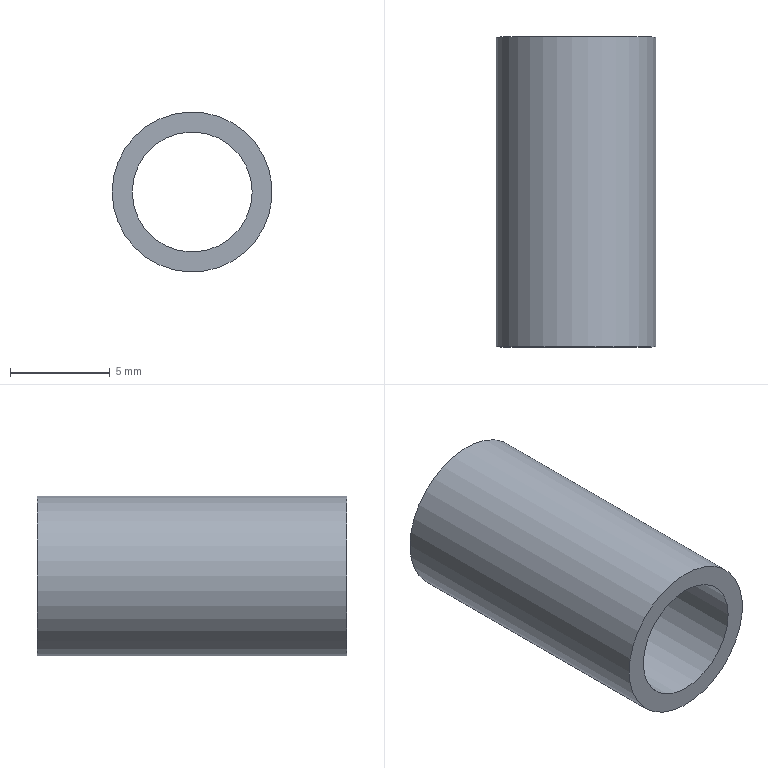Part | STEP file | 1-41.4 | 1 solid | 4 faces | box 8 x 15.5 x 8 mm | volume 340.863 mm3 | plane 2 | cylinder 2 | commonest cylinder face diameters 6 x1 8 x1
STEP:
#1=CARTESIAN_POINT('',(0.,0.,0.));
#2=DIRECTION('',(0.,0.,1.));
#3=DIRECTION('',(1.,0.,0.));
#4=AXIS2_PLACEMENT_3D('',#1,#2,#3);
#5=CARTESIAN_POINT('',(-4.,0.,0.));
#6=VERTEX_POINT('',#5);
#7=CARTESIAN_POINT('',(0.,0.,0.));
#8=DIRECTION('',(0.,1.,0.));
#9=DIRECTION('',(-1.,0.,0.));
#10=AXIS2_PLACEMENT_3D('',#7,#8,#9);
#11=CIRCLE('',#10,4.);
#12=CARTESIAN_POINT('',(1.072,0.,0.));
#13=DIRECTION('',(0.,1.,0.));
#14=DIRECTION('',(-1.,0.,0.));
#15=AXIS2_PLACEMENT_3D('',#12,#13,#14);
#16=PLANE('',#15);
#17=CARTESIAN_POINT('',(1.072,0.));
#18=DIRECTION('',(1.,0.));
#19=AXIS2_PLACEMENT_2D('',#17,#18);
#20=CIRCLE('',#19,4.);
#21=(GEOMETRIC_REPRESENTATION_CONTEXT(2)PARAMETRIC_REPRESENTATION_CONTEXT()REPRESENTATION_CONTEXT('',''));
#22=DEFINITIONAL_REPRESENTATION('',(#20),#21);
#23=PCURVE('',#16,#22);
#24=CARTESIAN_POINT('',(0.,0.,0.));
#25=DIRECTION('',(0.,-1.,0.));
#26=DIRECTION('',(-1.,0.,0.));
#27=AXIS2_PLACEMENT_3D('',#24,#25,#26);
#28=CYLINDRICAL_SURFACE('',#27,4.);
#29=CARTESIAN_POINT('',(6.283,0.));
#30=DIRECTION('',(-1.,0.));
#31=VECTOR('',#30,1.);
#32=LINE('',#29,#31);
#33=(GEOMETRIC_REPRESENTATION_CONTEXT(2)PARAMETRIC_REPRESENTATION_CONTEXT()REPRESENTATION_CONTEXT('',''));
#34=DEFINITIONAL_REPRESENTATION('',(#32),#33);
#35=PCURVE('',#28,#34);
#36=SURFACE_CURVE('',#11,(#23,#35),.PCURVE_S1.);
#37=EDGE_CURVE('',#6,#6,#36,.T.);
#38=ORIENTED_EDGE('',*,*,#37,.T.);
#39=EDGE_LOOP('',(#38));
#40=FACE_BOUND('',#39,.T.);
#41=CARTESIAN_POINT('',(-3.,0.,0.));
#42=VERTEX_POINT('',#41);
#43=CARTESIAN_POINT('',(0.,0.,0.));
#44=DIRECTION('',(0.,-1.,0.));
#45=DIRECTION('',(-1.,0.,0.));
#46=AXIS2_PLACEMENT_3D('',#43,#44,#45);
#47=CIRCLE('',#46,3.);
#48=CARTESIAN_POINT('',(4.072,0.));
#49=CARTESIAN_POINT('',(4.072,-5.196));
#50=CARTESIAN_POINT('',(-0.4282,-2.598));
#51=CARTESIAN_POINT('',(-4.928,0.));
#52=CARTESIAN_POINT('',(-0.4282,2.598));
#53=CARTESIAN_POINT('',(4.072,5.196));
#54=CARTESIAN_POINT('',(4.072,0.));
#55=(BOUNDED_CURVE()B_SPLINE_CURVE(2,(#48,#49,#50,#51,#52,#53,#54),.UNSPECIFIED.,.T.,.F.)B_SPLINE_CURVE_WITH_KNOTS((1,2,2,2,2,1),(-2.094,0.,2.094,4.189,6.283,8.378),.UNSPECIFIED.)CURVE()GEOMETRIC_REPRESENTATION_ITEM()RATIONAL_B_SPLINE_CURVE((1.,0.5,1.,0.5,1.,0.5,1.))REPRESENTATION_ITEM(''));
#56=(GEOMETRIC_REPRESENTATION_CONTEXT(2)PARAMETRIC_REPRESENTATION_CONTEXT()REPRESENTATION_CONTEXT('',''));
#57=DEFINITIONAL_REPRESENTATION('',(#55),#56);
#58=PCURVE('',#16,#57);
#59=CARTESIAN_POINT('',(0.,0.,0.));
#60=DIRECTION('',(0.,-1.,0.));
#61=DIRECTION('',(-1.,0.,0.));
#62=AXIS2_PLACEMENT_3D('',#59,#60,#61);
#63=CYLINDRICAL_SURFACE('',#62,3.);
#64=CARTESIAN_POINT('',(0.,0.));
#65=DIRECTION('',(1.,0.));
#66=VECTOR('',#65,1.);
#67=LINE('',#64,#66);
#68=(GEOMETRIC_REPRESENTATION_CONTEXT(2)PARAMETRIC_REPRESENTATION_CONTEXT()REPRESENTATION_CONTEXT('',''));
#69=DEFINITIONAL_REPRESENTATION('',(#67),#68);
#70=PCURVE('',#63,#69);
#71=SURFACE_CURVE('',#47,(#58,#70),.PCURVE_S1.);
#72=EDGE_CURVE('',#42,#42,#71,.T.);
#73=ORIENTED_EDGE('',*,*,#72,.T.);
#74=EDGE_LOOP('',(#73));
#75=FACE_BOUND('',#74,.T.);
#76=ADVANCED_FACE('',(#40,#75),#16,.T.);
#77=CARTESIAN_POINT('',(-4.,-15.5,0.));
#78=VERTEX_POINT('',#77);
#79=CARTESIAN_POINT('',(0.,-15.5,0.));
#80=DIRECTION('',(0.,1.,0.));
#81=DIRECTION('',(-1.,0.,0.));
#82=AXIS2_PLACEMENT_3D('',#79,#80,#81);
#83=CIRCLE('',#82,4.);
#84=CARTESIAN_POINT('',(1.072,-15.5,0.));
#85=DIRECTION('',(0.,1.,0.));
#86=DIRECTION('',(-1.,0.,0.));
#87=AXIS2_PLACEMENT_3D('',#84,#85,#86);
#88=PLANE('',#87);
#89=CARTESIAN_POINT('',(1.072,0.));
#90=DIRECTION('',(1.,0.));
#91=AXIS2_PLACEMENT_2D('',#89,#90);
#92=CIRCLE('',#91,4.);
#93=(GEOMETRIC_REPRESENTATION_CONTEXT(2)PARAMETRIC_REPRESENTATION_CONTEXT()REPRESENTATION_CONTEXT('',''));
#94=DEFINITIONAL_REPRESENTATION('',(#92),#93);
#95=PCURVE('',#88,#94);
#96=CARTESIAN_POINT('',(6.283,15.5));
#97=DIRECTION('',(-1.,0.));
#98=VECTOR('',#97,1.);
#99=LINE('',#96,#98);
#100=(GEOMETRIC_REPRESENTATION_CONTEXT(2)PARAMETRIC_REPRESENTATION_CONTEXT()REPRESENTATION_CONTEXT('',''));
#101=DEFINITIONAL_REPRESENTATION('',(#99),#100);
#102=PCURVE('',#28,#101);
#103=SURFACE_CURVE('',#83,(#95,#102),.PCURVE_S1.);
#104=EDGE_CURVE('',#78,#78,#103,.T.);
#105=ORIENTED_EDGE('',*,*,#104,.T.);
#106=EDGE_LOOP('',(#105));
#107=FACE_BOUND('',#106,.F.);
#108=CARTESIAN_POINT('',(-3.,-15.5,0.));
#109=VERTEX_POINT('',#108);
#110=CARTESIAN_POINT('',(0.,-15.5,0.));
#111=DIRECTION('',(0.,-1.,0.));
#112=DIRECTION('',(-1.,0.,0.));
#113=AXIS2_PLACEMENT_3D('',#110,#111,#112);
#114=CIRCLE('',#113,3.);
#115=CARTESIAN_POINT('',(4.072,0.));
#116=CARTESIAN_POINT('',(4.072,-5.196));
#117=CARTESIAN_POINT('',(-0.4282,-2.598));
#118=CARTESIAN_POINT('',(-4.928,0.));
#119=CARTESIAN_POINT('',(-0.4282,2.598));
#120=CARTESIAN_POINT('',(4.072,5.196));
#121=CARTESIAN_POINT('',(4.072,0.));
#122=(BOUNDED_CURVE()B_SPLINE_CURVE(2,(#115,#116,#117,#118,#119,#120,#121),.UNSPECIFIED.,.T.,.F.)B_SPLINE_CURVE_WITH_KNOTS((1,2,2,2,2,1),(-2.094,0.,2.094,4.189,6.283,8.378),.UNSPECIFIED.)CURVE()GEOMETRIC_REPRESENTATION_ITEM()RATIONAL_B_SPLINE_CURVE((1.,0.5,1.,0.5,1.,0.5,1.))REPRESENTATION_ITEM(''));
#123=(GEOMETRIC_REPRESENTATION_CONTEXT(2)PARAMETRIC_REPRESENTATION_CONTEXT()REPRESENTATION_CONTEXT('',''));
#124=DEFINITIONAL_REPRESENTATION('',(#122),#123);
#125=PCURVE('',#88,#124);
#126=CARTESIAN_POINT('',(0.,15.5));
#127=DIRECTION('',(1.,0.));
#128=VECTOR('',#127,1.);
#129=LINE('',#126,#128);
#130=(GEOMETRIC_REPRESENTATION_CONTEXT(2)PARAMETRIC_REPRESENTATION_CONTEXT()REPRESENTATION_CONTEXT('',''));
#131=DEFINITIONAL_REPRESENTATION('',(#129),#130);
#132=PCURVE('',#63,#131);
#133=SURFACE_CURVE('',#114,(#125,#132),.PCURVE_S1.);
#134=EDGE_CURVE('',#109,#109,#133,.T.);
#135=ORIENTED_EDGE('',*,*,#134,.T.);
#136=EDGE_LOOP('',(#135));
#137=FACE_BOUND('',#136,.F.);
#138=ADVANCED_FACE('',(#107,#137),#88,.F.);
#139=CARTESIAN_POINT('',(-4.,0.,0.));
#140=DIRECTION('',(0.,-1.,0.));
#141=VECTOR('',#140,1.);
#142=LINE('',#139,#141);
#143=CARTESIAN_POINT('',(6.283,0.));
#144=DIRECTION('',(0.,1.));
#145=VECTOR('',#144,1.);
#146=LINE('',#143,#145);
#147=(GEOMETRIC_REPRESENTATION_CONTEXT(2)PARAMETRIC_REPRESENTATION_CONTEXT()REPRESENTATION_CONTEXT('',''));
#148=DEFINITIONAL_REPRESENTATION('',(#146),#147);
#149=PCURVE('',#28,#148);
#150=CARTESIAN_POINT('',(0.,0.));
#151=DIRECTION('',(0.,1.));
#152=VECTOR('',#151,1.);
#153=LINE('',#150,#152);
#154=(GEOMETRIC_REPRESENTATION_CONTEXT(2)PARAMETRIC_REPRESENTATION_CONTEXT()REPRESENTATION_CONTEXT('',''));
#155=DEFINITIONAL_REPRESENTATION('',(#153),#154);
#156=PCURVE('',#28,#155);
#157=SEAM_CURVE('',#142,(#149,#156),.PCURVE_S1.);
#158=EDGE_CURVE('',#6,#78,#157,.T.);
#159=ORIENTED_EDGE('',*,*,#158,.T.);
#160=ORIENTED_EDGE('',*,*,#104,.T.);
#161=ORIENTED_EDGE('',*,*,#158,.F.);
#162=ORIENTED_EDGE('',*,*,#37,.F.);
#163=EDGE_LOOP('',(#159,#160,#161,#162));
#164=FACE_BOUND('',#163,.T.);
#165=ADVANCED_FACE('',(#164),#28,.T.);
#166=ORIENTED_EDGE('',*,*,#72,.T.);
#167=CARTESIAN_POINT('',(-3.,0.,0.));
#168=DIRECTION('',(0.,-1.,0.));
#169=VECTOR('',#168,1.);
#170=LINE('',#167,#169);
#171=CARTESIAN_POINT('',(6.283,0.));
#172=DIRECTION('',(0.,1.));
#173=VECTOR('',#172,1.);
#174=LINE('',#171,#173);
#175=(GEOMETRIC_REPRESENTATION_CONTEXT(2)PARAMETRIC_REPRESENTATION_CONTEXT()REPRESENTATION_CONTEXT('',''));
#176=DEFINITIONAL_REPRESENTATION('',(#174),#175);
#177=PCURVE('',#63,#176);
#178=CARTESIAN_POINT('',(0.,0.));
#179=DIRECTION('',(0.,1.));
#180=VECTOR('',#179,1.);
#181=LINE('',#178,#180);
#182=(GEOMETRIC_REPRESENTATION_CONTEXT(2)PARAMETRIC_REPRESENTATION_CONTEXT()REPRESENTATION_CONTEXT('',''));
#183=DEFINITIONAL_REPRESENTATION('',(#181),#182);
#184=PCURVE('',#63,#183);
#185=SEAM_CURVE('',#170,(#177,#184),.PCURVE_S1.);
#186=EDGE_CURVE('',#42,#109,#185,.T.);
#187=ORIENTED_EDGE('',*,*,#186,.T.);
#188=ORIENTED_EDGE('',*,*,#134,.F.);
#189=ORIENTED_EDGE('',*,*,#186,.F.);
#190=EDGE_LOOP('',(#166,#187,#188,#189));
#191=FACE_BOUND('',#190,.F.);
#192=ADVANCED_FACE('',(#191),#63,.F.);
#193=CLOSED_SHELL('',(#76,#138,#165,#192));
#194=MANIFOLD_SOLID_BREP('',#193);
#195=(LENGTH_UNIT()NAMED_UNIT(*)SI_UNIT(.MILLI.,.METRE.));
#196=UNCERTAINTY_MEASURE_WITH_UNIT(LENGTH_MEASURE(0.0000001),#195,'','');
#197=(NAMED_UNIT(*)PLANE_ANGLE_UNIT()SI_UNIT($,.RADIAN.));
#198=(NAMED_UNIT(*)SI_UNIT($,.STERADIAN.)SOLID_ANGLE_UNIT());
#199=(GEOMETRIC_REPRESENTATION_CONTEXT(3)GLOBAL_UNCERTAINTY_ASSIGNED_CONTEXT((#196))GLOBAL_UNIT_ASSIGNED_CONTEXT((#195,#197,#198))REPRESENTATION_CONTEXT('',''));
#200=ADVANCED_BREP_SHAPE_REPRESENTATION('',(#4,#194),#199);